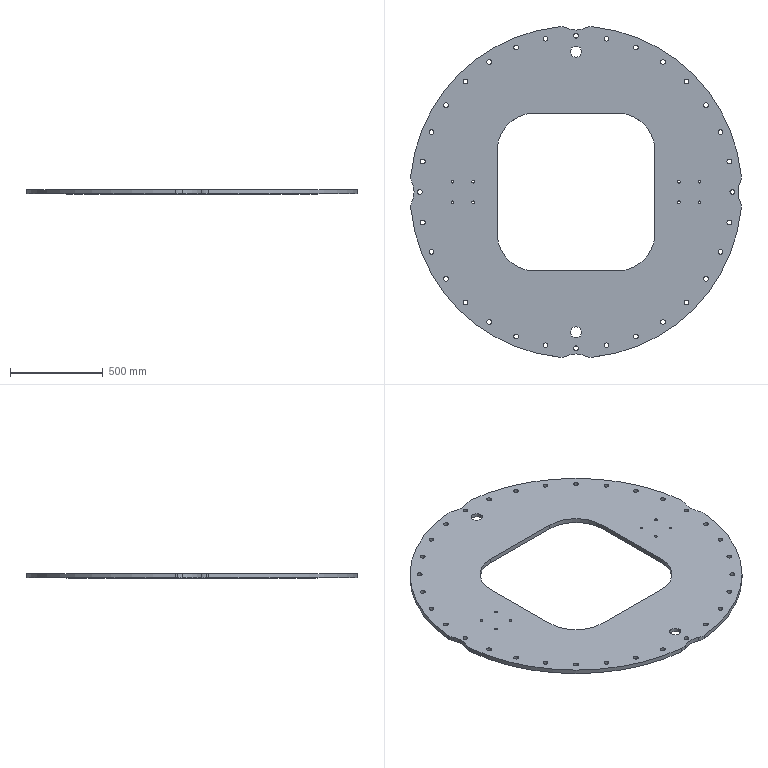Part | SolidWorks | features ICE 2, Extrusion 1 | 1 solid | 122 faces | box 1782 x 1782 x 25 mm | volume 40028246 mm3 | cylinder 114 | plane 8 | commonest cylinder face diameters 26 x64 14.5 x16 140 x10 245 x5 1350 x5 60 x4